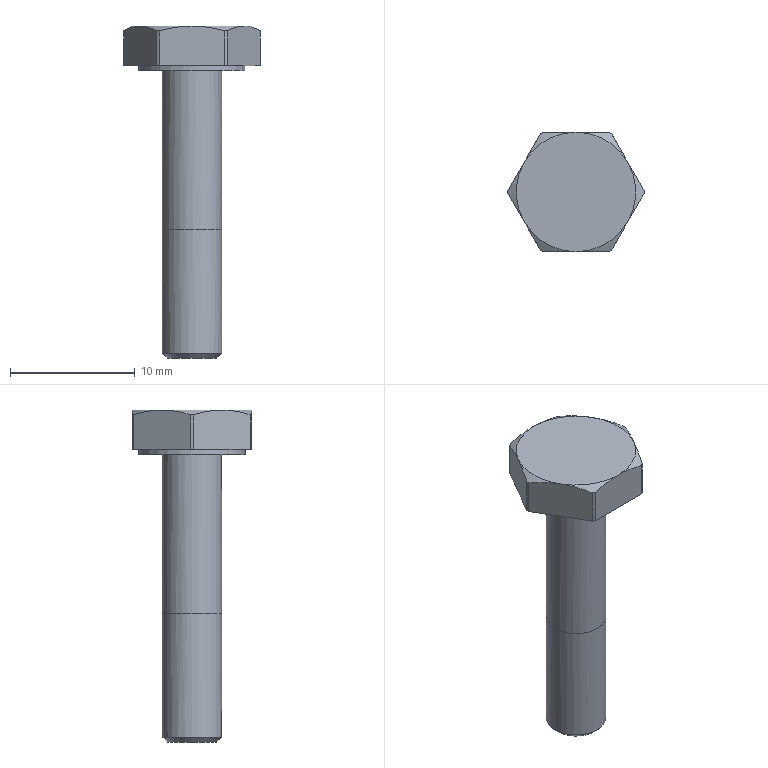Part | NX | features solid 2 | 1 solid | 26 faces | box 10.922 x 9.576 x 26.6 mm | volume 683.167 mm3 | plane 10 | cylinder 9 | cone 7 | commonest cylinder face diameters 10.922 x6 4.763 x2 8.509 x1
STEP:
#1=CARTESIAN_POINT('',(-2.381,0.,-3.581));
#2=VERTEX_POINT('',#1);
#3=CARTESIAN_POINT('',(0.,0.,-3.581));
#4=DIRECTION('',(0.,0.,-1.));
#5=DIRECTION('',(-1.,0.,0.));
#6=AXIS2_PLACEMENT_3D('',#3,#4,#5);
#7=CIRCLE('',#6,2.381);
#8=EDGE_CURVE('',#2,#2,#7,.T.);
#9=ORIENTED_EDGE('',*,*,#8,.T.);
#10=EDGE_LOOP('',(#9));
#11=FACE_BOUND('',#10,.T.);
#12=CARTESIAN_POINT('',(-2.381,0.,-16.281));
#13=VERTEX_POINT('',#12);
#14=CARTESIAN_POINT('',(-1.866,1.866,-16.281));
#15=CARTESIAN_POINT('',(-2.639,0.,-16.281));
#16=CARTESIAN_POINT('',(-1.866,-1.866,-16.281));
#17=CARTESIAN_POINT('',(0.,-2.639,-16.281));
#18=CARTESIAN_POINT('',(1.866,-1.866,-16.281));
#19=CARTESIAN_POINT('',(2.639,0.,-16.281));
#20=CARTESIAN_POINT('',(1.866,1.866,-16.281));
#21=CARTESIAN_POINT('',(0.,2.639,-16.281));
#22=CARTESIAN_POINT('',(-1.866,1.866,-16.281));
#23=CARTESIAN_POINT('',(-2.639,0.,-16.281));
#24=CARTESIAN_POINT('',(-1.866,-1.866,-16.281));
#25=B_SPLINE_CURVE_WITH_KNOTS('',3,(#14,#15,#16,#17,#18,#19,#20,#21,#22,#23,#24),.UNSPECIFIED.,.T.,.F.,(1,1,1,1,1,1,1,1,1,1,1,1,1,1,1),(-0.375,-0.25,-0.125,0.,0.125,0.25,0.375,0.5,0.625,0.75,0.875,1.,1.125,1.25,1.375),.UNSPECIFIED.);
#26=EDGE_CURVE('',#13,#13,#25,.T.);
#27=ORIENTED_EDGE('',*,*,#26,.T.);
#28=EDGE_LOOP('',(#27));
#29=FACE_BOUND('',#28,.T.);
#30=CARTESIAN_POINT('',(0.,0.,0.));
#31=DIRECTION('',(0.,0.,-1.));
#32=DIRECTION('',(-1.,0.,0.));
#33=AXIS2_PLACEMENT_3D('',#30,#31,#32);
#34=CYLINDRICAL_SURFACE('',#33,2.381);
#35=ADVANCED_FACE('',(#11,#29),#34,.T.);
#36=CARTESIAN_POINT('',(2.627,4.788,-3.175));
#37=VERTEX_POINT('',#36);
#38=CARTESIAN_POINT('',(2.833,4.669,-3.175));
#39=VERTEX_POINT('',#38);
#40=CARTESIAN_POINT('',(0.,0.,-3.175));
#41=DIRECTION('',(0.,0.,-1.));
#42=DIRECTION('',(-1.,0.,0.));
#43=AXIS2_PLACEMENT_3D('',#40,#41,#42);
#44=CIRCLE('',#43,5.461);
#45=EDGE_CURVE('',#37,#39,#44,.T.);
#46=ORIENTED_EDGE('',*,*,#45,.F.);
#47=CARTESIAN_POINT('',(2.627,4.788,-0.3886));
#48=VERTEX_POINT('',#47);
#49=CARTESIAN_POINT('',(2.627,4.788,0.));
#50=DIRECTION('',(0.,0.,-1.));
#51=VECTOR('',#50,1000.);
#52=LINE('',#49,#51);
#53=EDGE_CURVE('',#37,#48,#52,.F.);
#54=ORIENTED_EDGE('',*,*,#53,.T.);
#55=CARTESIAN_POINT('',(2.833,4.669,-0.3886));
#56=VERTEX_POINT('',#55);
#57=CARTESIAN_POINT('',(0.,0.,-0.3886));
#58=DIRECTION('',(0.,0.,-1.));
#59=DIRECTION('',(-1.,0.,0.));
#60=AXIS2_PLACEMENT_3D('',#57,#58,#59);
#61=CIRCLE('',#60,5.461);
#62=EDGE_CURVE('',#48,#56,#61,.T.);
#63=ORIENTED_EDGE('',*,*,#62,.T.);
#64=CARTESIAN_POINT('',(2.833,4.669,0.));
#65=DIRECTION('',(0.,0.,-1.));
#66=VECTOR('',#65,1000.);
#67=LINE('',#64,#66);
#68=EDGE_CURVE('',#56,#39,#67,.T.);
#69=ORIENTED_EDGE('',*,*,#68,.T.);
#70=EDGE_LOOP('',(#46,#54,#63,#69));
#71=FACE_BOUND('',#70,.T.);
#72=CARTESIAN_POINT('',(0.,0.,0.));
#73=DIRECTION('',(0.,0.,-1.));
#74=DIRECTION('',(-1.,0.,0.));
#75=AXIS2_PLACEMENT_3D('',#72,#73,#74);
#76=CYLINDRICAL_SURFACE('',#75,5.461);
#77=ADVANCED_FACE('',(#71),#76,.T.);
#78=CARTESIAN_POINT('',(-2.833,4.669,-0.3886));
#79=VERTEX_POINT('',#78);
#80=CARTESIAN_POINT('',(-2.627,4.788,-0.3886));
#81=VERTEX_POINT('',#80);
#82=CARTESIAN_POINT('',(0.,0.,-0.3886));
#83=DIRECTION('',(0.,0.,-1.));
#84=DIRECTION('',(-1.,0.,0.));
#85=AXIS2_PLACEMENT_3D('',#82,#83,#84);
#86=CIRCLE('',#85,5.461);
#87=EDGE_CURVE('',#79,#81,#86,.T.);
#88=ORIENTED_EDGE('',*,*,#87,.T.);
#89=CARTESIAN_POINT('',(-2.627,4.788,-3.175));
#90=VERTEX_POINT('',#89);
#91=CARTESIAN_POINT('',(-2.627,4.788,0.));
#92=DIRECTION('',(0.,0.,-1.));
#93=VECTOR('',#92,1000.);
#94=LINE('',#91,#93);
#95=EDGE_CURVE('',#81,#90,#94,.T.);
#96=ORIENTED_EDGE('',*,*,#95,.T.);
#97=CARTESIAN_POINT('',(-2.833,4.669,-3.175));
#98=VERTEX_POINT('',#97);
#99=CARTESIAN_POINT('',(0.,0.,-3.175));
#100=DIRECTION('',(0.,0.,-1.));
#101=DIRECTION('',(-1.,0.,0.));
#102=AXIS2_PLACEMENT_3D('',#99,#100,#101);
#103=CIRCLE('',#102,5.461);
#104=EDGE_CURVE('',#98,#90,#103,.T.);
#105=ORIENTED_EDGE('',*,*,#104,.F.);
#106=CARTESIAN_POINT('',(-2.833,4.669,0.));
#107=DIRECTION('',(0.,0.,-1.));
#108=VECTOR('',#107,1000.);
#109=LINE('',#106,#108);
#110=EDGE_CURVE('',#98,#79,#109,.F.);
#111=ORIENTED_EDGE('',*,*,#110,.T.);
#112=EDGE_LOOP('',(#88,#96,#105,#111));
#113=FACE_BOUND('',#112,.T.);
#114=CARTESIAN_POINT('',(0.,0.,0.));
#115=DIRECTION('',(0.,0.,-1.));
#116=DIRECTION('',(-1.,0.,0.));
#117=AXIS2_PLACEMENT_3D('',#114,#115,#116);
#118=CYLINDRICAL_SURFACE('',#117,5.461);
#119=ADVANCED_FACE('',(#113),#118,.T.);
#120=CARTESIAN_POINT('',(-5.46,-0.1193,-0.3886));
#121=VERTEX_POINT('',#120);
#122=CARTESIAN_POINT('',(-5.46,0.1193,-0.3886));
#123=VERTEX_POINT('',#122);
#124=CARTESIAN_POINT('',(0.,0.,-0.3886));
#125=DIRECTION('',(0.,0.,-1.));
#126=DIRECTION('',(-1.,0.,0.));
#127=AXIS2_PLACEMENT_3D('',#124,#125,#126);
#128=CIRCLE('',#127,5.461);
#129=EDGE_CURVE('',#121,#123,#128,.T.);
#130=ORIENTED_EDGE('',*,*,#129,.T.);
#131=CARTESIAN_POINT('',(-5.46,0.1193,-3.175));
#132=VERTEX_POINT('',#131);
#133=CARTESIAN_POINT('',(-5.46,0.1193,0.));
#134=DIRECTION('',(0.,0.,-1.));
#135=VECTOR('',#134,1000.);
#136=LINE('',#133,#135);
#137=EDGE_CURVE('',#123,#132,#136,.T.);
#138=ORIENTED_EDGE('',*,*,#137,.T.);
#139=CARTESIAN_POINT('',(-5.46,-0.1193,-3.175));
#140=VERTEX_POINT('',#139);
#141=CARTESIAN_POINT('',(0.,0.,-3.175));
#142=DIRECTION('',(0.,0.,-1.));
#143=DIRECTION('',(-1.,0.,0.));
#144=AXIS2_PLACEMENT_3D('',#141,#142,#143);
#145=CIRCLE('',#144,5.461);
#146=EDGE_CURVE('',#140,#132,#145,.T.);
#147=ORIENTED_EDGE('',*,*,#146,.F.);
#148=CARTESIAN_POINT('',(-5.46,-0.1193,0.));
#149=DIRECTION('',(0.,0.,-1.));
#150=VECTOR('',#149,1000.);
#151=LINE('',#148,#150);
#152=EDGE_CURVE('',#140,#121,#151,.F.);
#153=ORIENTED_EDGE('',*,*,#152,.T.);
#154=EDGE_LOOP('',(#130,#138,#147,#153));
#155=FACE_BOUND('',#154,.T.);
#156=CARTESIAN_POINT('',(0.,0.,0.));
#157=DIRECTION('',(0.,0.,-1.));
#158=DIRECTION('',(-1.,0.,0.));
#159=AXIS2_PLACEMENT_3D('',#156,#157,#158);
#160=CYLINDRICAL_SURFACE('',#159,5.461);
#161=ADVANCED_FACE('',(#155),#160,.T.);
#162=CARTESIAN_POINT('',(-2.627,-4.788,-0.3886));
#163=VERTEX_POINT('',#162);
#164=CARTESIAN_POINT('',(-2.833,-4.669,-0.3886));
#165=VERTEX_POINT('',#164);
#166=CARTESIAN_POINT('',(0.,0.,-0.3886));
#167=DIRECTION('',(0.,0.,-1.));
#168=DIRECTION('',(-1.,0.,0.));
#169=AXIS2_PLACEMENT_3D('',#166,#167,#168);
#170=CIRCLE('',#169,5.461);
#171=EDGE_CURVE('',#163,#165,#170,.T.);
#172=ORIENTED_EDGE('',*,*,#171,.T.);
#173=CARTESIAN_POINT('',(-2.833,-4.669,-3.175));
#174=VERTEX_POINT('',#173);
#175=CARTESIAN_POINT('',(-2.833,-4.669,0.));
#176=DIRECTION('',(0.,0.,-1.));
#177=VECTOR('',#176,1000.);
#178=LINE('',#175,#177);
#179=EDGE_CURVE('',#165,#174,#178,.T.);
#180=ORIENTED_EDGE('',*,*,#179,.T.);
#181=CARTESIAN_POINT('',(-2.627,-4.788,-3.175));
#182=VERTEX_POINT('',#181);
#183=CARTESIAN_POINT('',(0.,0.,-3.175));
#184=DIRECTION('',(0.,0.,-1.));
#185=DIRECTION('',(-1.,0.,0.));
#186=AXIS2_PLACEMENT_3D('',#183,#184,#185);
#187=CIRCLE('',#186,5.461);
#188=EDGE_CURVE('',#182,#174,#187,.T.);
#189=ORIENTED_EDGE('',*,*,#188,.F.);
#190=CARTESIAN_POINT('',(-2.627,-4.788,0.));
#191=DIRECTION('',(0.,0.,-1.));
#192=VECTOR('',#191,1000.);
#193=LINE('',#190,#192);
#194=EDGE_CURVE('',#182,#163,#193,.F.);
#195=ORIENTED_EDGE('',*,*,#194,.T.);
#196=EDGE_LOOP('',(#172,#180,#189,#195));
#197=FACE_BOUND('',#196,.T.);
#198=CARTESIAN_POINT('',(0.,0.,0.));
#199=DIRECTION('',(0.,0.,-1.));
#200=DIRECTION('',(-1.,0.,0.));
#201=AXIS2_PLACEMENT_3D('',#198,#199,#200);
#202=CYLINDRICAL_SURFACE('',#201,5.461);
#203=ADVANCED_FACE('',(#197),#202,.T.);
#204=CARTESIAN_POINT('',(2.833,-4.669,-0.3886));
#205=VERTEX_POINT('',#204);
#206=CARTESIAN_POINT('',(2.627,-4.788,-0.3886));
#207=VERTEX_POINT('',#206);
#208=CARTESIAN_POINT('',(0.,0.,-0.3886));
#209=DIRECTION('',(0.,0.,-1.));
#210=DIRECTION('',(-1.,0.,0.));
#211=AXIS2_PLACEMENT_3D('',#208,#209,#210);
#212=CIRCLE('',#211,5.461);
#213=EDGE_CURVE('',#205,#207,#212,.T.);
#214=ORIENTED_EDGE('',*,*,#213,.T.);
#215=CARTESIAN_POINT('',(2.627,-4.788,-3.175));
#216=VERTEX_POINT('',#215);
#217=CARTESIAN_POINT('',(2.627,-4.788,0.));
#218=DIRECTION('',(0.,0.,-1.));
#219=VECTOR('',#218,1000.);
#220=LINE('',#217,#219);
#221=EDGE_CURVE('',#207,#216,#220,.T.);
#222=ORIENTED_EDGE('',*,*,#221,.T.);
#223=CARTESIAN_POINT('',(2.833,-4.669,-3.175));
#224=VERTEX_POINT('',#223);
#225=CARTESIAN_POINT('',(0.,0.,-3.175));
#226=DIRECTION('',(0.,0.,-1.));
#227=DIRECTION('',(-1.,0.,0.));
#228=AXIS2_PLACEMENT_3D('',#225,#226,#227);
#229=CIRCLE('',#228,5.461);
#230=EDGE_CURVE('',#224,#216,#229,.T.);
#231=ORIENTED_EDGE('',*,*,#230,.F.);
#232=CARTESIAN_POINT('',(2.833,-4.669,0.));
#233=DIRECTION('',(0.,0.,-1.));
#234=VECTOR('',#233,1000.);
#235=LINE('',#232,#234);
#236=EDGE_CURVE('',#224,#205,#235,.F.);
#237=ORIENTED_EDGE('',*,*,#236,.T.);
#238=EDGE_LOOP('',(#214,#222,#231,#237));
#239=FACE_BOUND('',#238,.T.);
#240=CARTESIAN_POINT('',(0.,0.,0.));
#241=DIRECTION('',(0.,0.,-1.));
#242=DIRECTION('',(-1.,0.,0.));
#243=AXIS2_PLACEMENT_3D('',#240,#241,#242);
#244=CYLINDRICAL_SURFACE('',#243,5.461);
#245=ADVANCED_FACE('',(#239),#244,.T.);
#246=ORIENTED_EDGE('',*,*,#62,.F.);
#247=CARTESIAN_POINT('',(0.,4.788,0.));
#248=VERTEX_POINT('',#247);
#249=CARTESIAN_POINT('',(0.,4.788,0.));
#250=CARTESIAN_POINT('',(0.8868,4.788,0.));
#251=CARTESIAN_POINT('',(1.776,4.788,-0.1525));
#252=CARTESIAN_POINT('',(2.627,4.788,-0.3886));
#253=B_SPLINE_CURVE_WITH_KNOTS('',3,(#249,#250,#251,#252),.UNSPECIFIED.,.F.,.F.,(4,4),(0.007722,0.01038),.UNSPECIFIED.);
#254=EDGE_CURVE('',#48,#248,#253,.F.);
#255=ORIENTED_EDGE('',*,*,#254,.T.);
#256=CARTESIAN_POINT('',(4.146,2.394,0.));
#257=VERTEX_POINT('',#256);
#258=CARTESIAN_POINT('',(0.,0.,0.));
#259=DIRECTION('',(0.,0.,-1.));
#260=DIRECTION('',(-1.,0.,0.));
#261=AXIS2_PLACEMENT_3D('',#258,#259,#260);
#262=CIRCLE('',#261,4.788);
#263=EDGE_CURVE('',#248,#257,#262,.T.);
#264=ORIENTED_EDGE('',*,*,#263,.T.);
#265=CARTESIAN_POINT('',(4.146,2.394,0.));
#266=CARTESIAN_POINT('',(3.703,3.163,0.));
#267=CARTESIAN_POINT('',(3.262,3.925,-0.1503));
#268=CARTESIAN_POINT('',(2.833,4.669,-0.3886));
#269=B_SPLINE_CURVE_WITH_KNOTS('',3,(#265,#266,#267,#268),.UNSPECIFIED.,.F.,.F.,(4,4),(0.002655,0.005296),.UNSPECIFIED.);
#270=EDGE_CURVE('',#257,#56,#269,.T.);
#271=ORIENTED_EDGE('',*,*,#270,.T.);
#272=EDGE_LOOP('',(#246,#255,#264,#271));
#273=FACE_BOUND('',#272,.T.);
#274=CARTESIAN_POINT('',(0.,0.,-0.3886));
#275=DIRECTION('',(0.,0.,-1.));
#276=DIRECTION('',(-1.,0.,0.));
#277=AXIS2_PLACEMENT_3D('',#274,#275,#276);
#278=CONICAL_SURFACE('',#277,5.461,1.047);
#279=ADVANCED_FACE('',(#273),#278,.T.);
#280=CARTESIAN_POINT('',(-4.146,2.394,0.));
#281=VERTEX_POINT('',#280);
#282=CARTESIAN_POINT('',(0.,0.,0.));
#283=DIRECTION('',(0.,0.,-1.));
#284=DIRECTION('',(-1.,0.,0.));
#285=AXIS2_PLACEMENT_3D('',#282,#283,#284);
#286=CIRCLE('',#285,4.788);
#287=EDGE_CURVE('',#281,#248,#286,.T.);
#288=ORIENTED_EDGE('',*,*,#287,.T.);
#289=CARTESIAN_POINT('',(-2.627,4.788,-0.3886));
#290=CARTESIAN_POINT('',(-1.77,4.788,-0.1508));
#291=CARTESIAN_POINT('',(-0.8866,4.788,0.));
#292=CARTESIAN_POINT('',(0.,4.788,0.));
#293=B_SPLINE_CURVE_WITH_KNOTS('',3,(#289,#290,#291,#292),.UNSPECIFIED.,.F.,.F.,(4,4),(0.005068,0.007722),.UNSPECIFIED.);
#294=EDGE_CURVE('',#248,#81,#293,.F.);
#295=ORIENTED_EDGE('',*,*,#294,.T.);
#296=ORIENTED_EDGE('',*,*,#87,.F.);
#297=CARTESIAN_POINT('',(-2.833,4.669,-0.3886));
#298=CARTESIAN_POINT('',(-3.264,3.923,-0.1495));
#299=CARTESIAN_POINT('',(-3.7,3.167,0.));
#300=CARTESIAN_POINT('',(-4.146,2.394,0.));
#301=B_SPLINE_CURVE_WITH_KNOTS('',3,(#297,#298,#299,#300),.UNSPECIFIED.,.F.,.F.,(4,4),(0.00000074,0.002655),.UNSPECIFIED.);
#302=EDGE_CURVE('',#79,#281,#301,.T.);
#303=ORIENTED_EDGE('',*,*,#302,.T.);
#304=EDGE_LOOP('',(#288,#295,#296,#303));
#305=FACE_BOUND('',#304,.T.);
#306=CARTESIAN_POINT('',(0.,0.,-0.3886));
#307=DIRECTION('',(0.,0.,-1.));
#308=DIRECTION('',(-1.,0.,0.));
#309=AXIS2_PLACEMENT_3D('',#306,#307,#308);
#310=CONICAL_SURFACE('',#309,5.461,1.047);
#311=ADVANCED_FACE('',(#305),#310,.T.);
#312=CARTESIAN_POINT('',(-4.146,-2.394,0.));
#313=VERTEX_POINT('',#312);
#314=CARTESIAN_POINT('',(0.,0.,0.));
#315=DIRECTION('',(0.,0.,-1.));
#316=DIRECTION('',(-1.,0.,0.));
#317=AXIS2_PLACEMENT_3D('',#314,#315,#316);
#318=CIRCLE('',#317,4.788);
#319=EDGE_CURVE('',#313,#281,#318,.T.);
#320=ORIENTED_EDGE('',*,*,#319,.T.);
#321=CARTESIAN_POINT('',(-4.146,2.394,0.));
#322=CARTESIAN_POINT('',(-4.59,1.625,0.));
#323=CARTESIAN_POINT('',(-5.031,0.8625,-0.1503));
#324=CARTESIAN_POINT('',(-5.46,0.1193,-0.3886));
#325=B_SPLINE_CURVE_WITH_KNOTS('',3,(#321,#322,#323,#324),.UNSPECIFIED.,.F.,.F.,(4,4),(0.002655,0.005296),.UNSPECIFIED.);
#326=EDGE_CURVE('',#281,#123,#325,.T.);
#327=ORIENTED_EDGE('',*,*,#326,.T.);
#328=ORIENTED_EDGE('',*,*,#129,.F.);
#329=CARTESIAN_POINT('',(-5.46,-0.1193,-0.3886));
#330=CARTESIAN_POINT('',(-5.029,-0.8651,-0.1495));
#331=CARTESIAN_POINT('',(-4.593,-1.621,0.));
#332=CARTESIAN_POINT('',(-4.146,-2.394,0.));
#333=B_SPLINE_CURVE_WITH_KNOTS('',3,(#329,#330,#331,#332),.UNSPECIFIED.,.F.,.F.,(4,4),(0.00000074,0.002655),.UNSPECIFIED.);
#334=EDGE_CURVE('',#121,#313,#333,.T.);
#335=ORIENTED_EDGE('',*,*,#334,.T.);
#336=EDGE_LOOP('',(#320,#327,#328,#335));
#337=FACE_BOUND('',#336,.T.);
#338=CARTESIAN_POINT('',(0.,0.,-0.3886));
#339=DIRECTION('',(0.,0.,-1.));
#340=DIRECTION('',(-1.,0.,0.));
#341=AXIS2_PLACEMENT_3D('',#338,#339,#340);
#342=CONICAL_SURFACE('',#341,5.461,1.047);
#343=ADVANCED_FACE('',(#337),#342,.T.);
#344=CARTESIAN_POINT('',(0.,-4.788,0.));
#345=VERTEX_POINT('',#344);
#346=CARTESIAN_POINT('',(0.,0.,0.));
#347=DIRECTION('',(0.,0.,-1.));
#348=DIRECTION('',(-1.,0.,0.));
#349=AXIS2_PLACEMENT_3D('',#346,#347,#348);
#350=CIRCLE('',#349,4.788);
#351=EDGE_CURVE('',#345,#313,#350,.T.);
#352=ORIENTED_EDGE('',*,*,#351,.T.);
#353=CARTESIAN_POINT('',(-4.146,-2.394,0.));
#354=CARTESIAN_POINT('',(-3.703,-3.163,0.));
#355=CARTESIAN_POINT('',(-3.262,-3.925,-0.1503));
#356=CARTESIAN_POINT('',(-2.833,-4.669,-0.3886));
#357=B_SPLINE_CURVE_WITH_KNOTS('',3,(#353,#354,#355,#356),.UNSPECIFIED.,.F.,.F.,(4,4),(0.002655,0.005296),.UNSPECIFIED.);
#358=EDGE_CURVE('',#313,#165,#357,.T.);
#359=ORIENTED_EDGE('',*,*,#358,.T.);
#360=ORIENTED_EDGE('',*,*,#171,.F.);
#361=CARTESIAN_POINT('',(-2.627,-4.788,-0.3886));
#362=CARTESIAN_POINT('',(-1.77,-4.788,-0.1508));
#363=CARTESIAN_POINT('',(-0.8866,-4.788,0.));
#364=CARTESIAN_POINT('',(0.,-4.788,0.));
#365=B_SPLINE_CURVE_WITH_KNOTS('',3,(#361,#362,#363,#364),.UNSPECIFIED.,.F.,.F.,(4,4),(0.005068,0.007722),.UNSPECIFIED.);
#366=EDGE_CURVE('',#163,#345,#365,.T.);
#367=ORIENTED_EDGE('',*,*,#366,.T.);
#368=EDGE_LOOP('',(#352,#359,#360,#367));
#369=FACE_BOUND('',#368,.T.);
#370=CARTESIAN_POINT('',(0.,0.,-0.3886));
#371=DIRECTION('',(0.,0.,-1.));
#372=DIRECTION('',(-1.,0.,0.));
#373=AXIS2_PLACEMENT_3D('',#370,#371,#372);
#374=CONICAL_SURFACE('',#373,5.461,1.047);
#375=ADVANCED_FACE('',(#369),#374,.T.);
#376=CARTESIAN_POINT('',(4.146,-2.394,0.));
#377=VERTEX_POINT('',#376);
#378=CARTESIAN_POINT('',(0.,0.,0.));
#379=DIRECTION('',(0.,0.,-1.));
#380=DIRECTION('',(-1.,0.,0.));
#381=AXIS2_PLACEMENT_3D('',#378,#379,#380);
#382=CIRCLE('',#381,4.788);
#383=EDGE_CURVE('',#377,#345,#382,.T.);
#384=ORIENTED_EDGE('',*,*,#383,.T.);
#385=CARTESIAN_POINT('',(0.,-4.788,0.));
#386=CARTESIAN_POINT('',(0.8868,-4.788,0.));
#387=CARTESIAN_POINT('',(1.776,-4.788,-0.1525));
#388=CARTESIAN_POINT('',(2.627,-4.788,-0.3886));
#389=B_SPLINE_CURVE_WITH_KNOTS('',3,(#385,#386,#387,#388),.UNSPECIFIED.,.F.,.F.,(4,4),(0.007722,0.01038),.UNSPECIFIED.);
#390=EDGE_CURVE('',#345,#207,#389,.T.);
#391=ORIENTED_EDGE('',*,*,#390,.T.);
#392=ORIENTED_EDGE('',*,*,#213,.F.);
#393=CARTESIAN_POINT('',(2.833,-4.669,-0.3886));
#394=CARTESIAN_POINT('',(3.264,-3.923,-0.1495));
#395=CARTESIAN_POINT('',(3.7,-3.167,0.));
#396=CARTESIAN_POINT('',(4.146,-2.394,0.));
#397=B_SPLINE_CURVE_WITH_KNOTS('',3,(#393,#394,#395,#396),.UNSPECIFIED.,.F.,.F.,(4,4),(0.00000074,0.002655),.UNSPECIFIED.);
#398=EDGE_CURVE('',#205,#377,#397,.T.);
#399=ORIENTED_EDGE('',*,*,#398,.T.);
#400=EDGE_LOOP('',(#384,#391,#392,#399));
#401=FACE_BOUND('',#400,.T.);
#402=CARTESIAN_POINT('',(0.,0.,-0.3886));
#403=DIRECTION('',(0.,0.,-1.));
#404=DIRECTION('',(-1.,0.,0.));
#405=AXIS2_PLACEMENT_3D('',#402,#403,#404);
#406=CONICAL_SURFACE('',#405,5.461,1.047);
#407=ADVANCED_FACE('',(#401),#406,.T.);
#408=ORIENTED_EDGE('',*,*,#104,.T.);
#409=CARTESIAN_POINT('',(4.255,4.788,-3.175));
#410=DIRECTION('',(1.,0.,0.));
#411=VECTOR('',#410,1000.);
#412=LINE('',#409,#411);
#413=EDGE_CURVE('',#90,#37,#412,.T.);
#414=ORIENTED_EDGE('',*,*,#413,.T.);
#415=ORIENTED_EDGE('',*,*,#45,.T.);
#416=CARTESIAN_POINT('',(5.46,0.1193,-3.175));
#417=VERTEX_POINT('',#416);
#418=CARTESIAN_POINT('',(5.21,0.5517,-3.175));
#419=DIRECTION('',(0.5,-0.866,0.));
#420=VECTOR('',#419,1000.);
#421=LINE('',#418,#420);
#422=EDGE_CURVE('',#39,#417,#421,.T.);
#423=ORIENTED_EDGE('',*,*,#422,.T.);
#424=CARTESIAN_POINT('',(5.46,-0.1193,-3.175));
#425=VERTEX_POINT('',#424);
#426=CARTESIAN_POINT('',(0.,0.,-3.175));
#427=DIRECTION('',(0.,0.,-1.));
#428=DIRECTION('',(-1.,0.,0.));
#429=AXIS2_PLACEMENT_3D('',#426,#427,#428);
#430=CIRCLE('',#429,5.461);
#431=EDGE_CURVE('',#417,#425,#430,.T.);
#432=ORIENTED_EDGE('',*,*,#431,.T.);
#433=CARTESIAN_POINT('',(5.21,-0.5517,-3.175));
#434=DIRECTION('',(-0.5,-0.866,0.));
#435=VECTOR('',#434,1000.);
#436=LINE('',#433,#435);
#437=EDGE_CURVE('',#425,#224,#436,.T.);
#438=ORIENTED_EDGE('',*,*,#437,.T.);
#439=ORIENTED_EDGE('',*,*,#230,.T.);
#440=CARTESIAN_POINT('',(4.255,-4.788,-3.175));
#441=DIRECTION('',(-1.,0.,0.));
#442=VECTOR('',#441,1000.);
#443=LINE('',#440,#442);
#444=EDGE_CURVE('',#216,#182,#443,.T.);
#445=ORIENTED_EDGE('',*,*,#444,.T.);
#446=ORIENTED_EDGE('',*,*,#188,.T.);
#447=CARTESIAN_POINT('',(-3.083,-4.236,-3.175));
#448=DIRECTION('',(-0.5,0.866,0.));
#449=VECTOR('',#448,1000.);
#450=LINE('',#447,#449);
#451=EDGE_CURVE('',#174,#140,#450,.T.);
#452=ORIENTED_EDGE('',*,*,#451,.T.);
#453=ORIENTED_EDGE('',*,*,#146,.T.);
#454=CARTESIAN_POINT('',(-3.083,4.236,-3.175));
#455=DIRECTION('',(0.5,0.866,0.));
#456=VECTOR('',#455,1000.);
#457=LINE('',#454,#456);
#458=EDGE_CURVE('',#132,#98,#457,.T.);
#459=ORIENTED_EDGE('',*,*,#458,.T.);
#460=EDGE_LOOP('',(#408,#414,#415,#423,#432,#438,#439,#445,#446,#452,#453,#459));
#461=FACE_BOUND('',#460,.T.);
#462=CARTESIAN_POINT('',(-4.255,0.,-3.175));
#463=VERTEX_POINT('',#462);
#464=CARTESIAN_POINT('',(0.,0.,-3.175));
#465=DIRECTION('',(0.,0.,-1.));
#466=DIRECTION('',(-1.,0.,0.));
#467=AXIS2_PLACEMENT_3D('',#464,#465,#466);
#468=CIRCLE('',#467,4.255);
#469=EDGE_CURVE('',#463,#463,#468,.T.);
#470=ORIENTED_EDGE('',*,*,#469,.F.);
#471=EDGE_LOOP('',(#470));
#472=FACE_BOUND('',#471,.T.);
#473=CARTESIAN_POINT('',(4.255,0.,-3.175));
#474=DIRECTION('',(0.,0.,-1.));
#475=DIRECTION('',(-1.,0.,0.));
#476=AXIS2_PLACEMENT_3D('',#473,#474,#475);
#477=PLANE('',#476);
#478=ADVANCED_FACE('',(#461,#472),#477,.T.);
#479=CARTESIAN_POINT('',(5.46,0.1193,-0.3886));
#480=VERTEX_POINT('',#479);
#481=CARTESIAN_POINT('',(5.46,-0.1193,-0.3886));
#482=VERTEX_POINT('',#481);
#483=CARTESIAN_POINT('',(0.,0.,-0.3886));
#484=DIRECTION('',(0.,0.,-1.));
#485=DIRECTION('',(-1.,0.,0.));
#486=AXIS2_PLACEMENT_3D('',#483,#484,#485);
#487=CIRCLE('',#486,5.461);
#488=EDGE_CURVE('',#480,#482,#487,.T.);
#489=ORIENTED_EDGE('',*,*,#488,.T.);
#490=CARTESIAN_POINT('',(5.46,-0.1193,0.));
#491=DIRECTION('',(0.,0.,-1.));
#492=VECTOR('',#491,1000.);
#493=LINE('',#490,#492);
#494=EDGE_CURVE('',#482,#425,#493,.T.);
#495=ORIENTED_EDGE('',*,*,#494,.T.);
#496=ORIENTED_EDGE('',*,*,#431,.F.);
#497=CARTESIAN_POINT('',(5.46,0.1193,0.));
#498=DIRECTION('',(0.,0.,-1.));
#499=VECTOR('',#498,1000.);
#500=LINE('',#497,#499);
#501=EDGE_CURVE('',#417,#480,#500,.F.);
#502=ORIENTED_EDGE('',*,*,#501,.T.);
#503=EDGE_LOOP('',(#489,#495,#496,#502));
#504=FACE_BOUND('',#503,.T.);
#505=CARTESIAN_POINT('',(0.,0.,0.));
#506=DIRECTION('',(0.,0.,-1.));
#507=DIRECTION('',(-1.,0.,0.));
#508=AXIS2_PLACEMENT_3D('',#505,#506,#507);
#509=CYLINDRICAL_SURFACE('',#508,5.461);
#510=ADVANCED_FACE('',(#504),#509,.T.);
#511=CARTESIAN_POINT('',(0.,0.,0.));
#512=DIRECTION('',(0.,0.,-1.));
#513=DIRECTION('',(-1.,0.,0.));
#514=AXIS2_PLACEMENT_3D('',#511,#512,#513);
#515=CIRCLE('',#514,4.788);
#516=EDGE_CURVE('',#257,#377,#515,.T.);
#517=ORIENTED_EDGE('',*,*,#516,.T.);
#518=CARTESIAN_POINT('',(4.146,-2.394,0.));
#519=CARTESIAN_POINT('',(4.59,-1.625,0.));
#520=CARTESIAN_POINT('',(5.031,-0.8625,-0.1503));
#521=CARTESIAN_POINT('',(5.46,-0.1193,-0.3886));
#522=B_SPLINE_CURVE_WITH_KNOTS('',3,(#518,#519,#520,#521),.UNSPECIFIED.,.F.,.F.,(4,4),(0.002655,0.005296),.UNSPECIFIED.);
#523=EDGE_CURVE('',#377,#482,#522,.T.);
#524=ORIENTED_EDGE('',*,*,#523,.T.);
#525=ORIENTED_EDGE('',*,*,#488,.F.);
#526=CARTESIAN_POINT('',(5.46,0.1193,-0.3886));
#527=CARTESIAN_POINT('',(5.029,0.8651,-0.1495));
#528=CARTESIAN_POINT('',(4.593,1.621,0.));
#529=CARTESIAN_POINT('',(4.146,2.394,0.));
#530=B_SPLINE_CURVE_WITH_KNOTS('',3,(#526,#527,#528,#529),.UNSPECIFIED.,.F.,.F.,(4,4),(0.00000074,0.002655),.UNSPECIFIED.);
#531=EDGE_CURVE('',#480,#257,#530,.T.);
#532=ORIENTED_EDGE('',*,*,#531,.T.);
#533=EDGE_LOOP('',(#517,#524,#525,#532));
#534=FACE_BOUND('',#533,.T.);
#535=CARTESIAN_POINT('',(0.,0.,-0.3886));
#536=DIRECTION('',(0.,0.,-1.));
#537=DIRECTION('',(-1.,0.,0.));
#538=AXIS2_PLACEMENT_3D('',#535,#536,#537);
#539=CONICAL_SURFACE('',#538,5.461,1.047);
#540=ADVANCED_FACE('',(#534),#539,.T.);
#541=ORIENTED_EDGE('',*,*,#287,.F.);
#542=ORIENTED_EDGE('',*,*,#319,.F.);
#543=ORIENTED_EDGE('',*,*,#351,.F.);
#544=ORIENTED_EDGE('',*,*,#383,.F.);
#545=ORIENTED_EDGE('',*,*,#516,.F.);
#546=ORIENTED_EDGE('',*,*,#263,.F.);
#547=EDGE_LOOP('',(#541,#542,#543,#544,#545,#546));
#548=FACE_BOUND('',#547,.T.);
#549=CARTESIAN_POINT('',(4.788,0.,0.));
#550=DIRECTION('',(0.,0.,1.));
#551=DIRECTION('',(1.,0.,0.));
#552=AXIS2_PLACEMENT_3D('',#549,#550,#551);
#553=PLANE('',#552);
#554=ADVANCED_FACE('',(#548),#553,.T.);
#555=CARTESIAN_POINT('',(-2.,0.,-26.6));
#556=VERTEX_POINT('',#555);
#557=CARTESIAN_POINT('',(0.,0.,-26.6));
#558=DIRECTION('',(0.,0.,-1.));
#559=DIRECTION('',(-1.,0.,0.));
#560=AXIS2_PLACEMENT_3D('',#557,#558,#559);
#561=CIRCLE('',#560,2.);
#562=EDGE_CURVE('',#556,#556,#561,.T.);
#563=ORIENTED_EDGE('',*,*,#562,.T.);
#564=EDGE_LOOP('',(#563));
#565=FACE_BOUND('',#564,.T.);
#566=CARTESIAN_POINT('',(0.,0.,-26.6));
#567=DIRECTION('',(0.,0.,-1.));
#568=DIRECTION('',(-1.,0.,0.));
#569=AXIS2_PLACEMENT_3D('',#566,#567,#568);
#570=PLANE('',#569);
#571=ADVANCED_FACE('',(#565),#570,.T.);
#572=CARTESIAN_POINT('',(-2.381,0.,-26.219));
#573=VERTEX_POINT('',#572);
#574=CARTESIAN_POINT('',(0.,0.,-26.219));
#575=DIRECTION('',(0.,0.,-1.));
#576=DIRECTION('',(-1.,0.,0.));
#577=AXIS2_PLACEMENT_3D('',#574,#575,#576);
#578=CIRCLE('',#577,2.381);
#579=EDGE_CURVE('',#573,#573,#578,.T.);
#580=ORIENTED_EDGE('',*,*,#579,.T.);
#581=EDGE_LOOP('',(#580));
#582=FACE_BOUND('',#581,.T.);
#583=ORIENTED_EDGE('',*,*,#562,.F.);
#584=EDGE_LOOP('',(#583));
#585=FACE_BOUND('',#584,.T.);
#586=CARTESIAN_POINT('',(0.,0.,-26.6));
#587=DIRECTION('',(0.,0.,1.));
#588=DIRECTION('',(1.,0.,0.));
#589=AXIS2_PLACEMENT_3D('',#586,#587,#588);
#590=CONICAL_SURFACE('',#589,2.,0.7854);
#591=ADVANCED_FACE('',(#582,#585),#590,.T.);
#592=ORIENTED_EDGE('',*,*,#26,.F.);
#593=EDGE_LOOP('',(#592));
#594=FACE_BOUND('',#593,.T.);
#595=ORIENTED_EDGE('',*,*,#579,.F.);
#596=EDGE_LOOP('',(#595));
#597=FACE_BOUND('',#596,.T.);
#598=CARTESIAN_POINT('',(0.,0.,0.));
#599=DIRECTION('',(0.,0.,-1.));
#600=DIRECTION('',(-1.,0.,0.));
#601=AXIS2_PLACEMENT_3D('',#598,#599,#600);
#602=CYLINDRICAL_SURFACE('',#601,2.381);
#603=ADVANCED_FACE('',(#594,#597),#602,.T.);
#604=CARTESIAN_POINT('',(-4.255,0.,-3.581));
#605=VERTEX_POINT('',#604);
#606=CARTESIAN_POINT('',(0.,0.,-3.581));
#607=DIRECTION('',(0.,0.,-1.));
#608=DIRECTION('',(-1.,0.,0.));
#609=AXIS2_PLACEMENT_3D('',#606,#607,#608);
#610=CIRCLE('',#609,4.255);
#611=EDGE_CURVE('',#605,#605,#610,.T.);
#612=ORIENTED_EDGE('',*,*,#611,.T.);
#613=EDGE_LOOP('',(#612));
#614=FACE_BOUND('',#613,.T.);
#615=ORIENTED_EDGE('',*,*,#8,.F.);
#616=EDGE_LOOP('',(#615));
#617=FACE_BOUND('',#616,.T.);
#618=CARTESIAN_POINT('',(2.381,0.,-3.581));
#619=DIRECTION('',(0.,0.,-1.));
#620=DIRECTION('',(-1.,0.,0.));
#621=AXIS2_PLACEMENT_3D('',#618,#619,#620);
#622=PLANE('',#621);
#623=ADVANCED_FACE('',(#614,#617),#622,.T.);
#624=ORIENTED_EDGE('',*,*,#469,.T.);
#625=EDGE_LOOP('',(#624));
#626=FACE_BOUND('',#625,.T.);
#627=ORIENTED_EDGE('',*,*,#611,.F.);
#628=EDGE_LOOP('',(#627));
#629=FACE_BOUND('',#628,.T.);
#630=CARTESIAN_POINT('',(0.,0.,0.));
#631=DIRECTION('',(0.,0.,-1.));
#632=DIRECTION('',(-1.,0.,0.));
#633=AXIS2_PLACEMENT_3D('',#630,#631,#632);
#634=CYLINDRICAL_SURFACE('',#633,4.255);
#635=ADVANCED_FACE('',(#626,#629),#634,.T.);
#636=ORIENTED_EDGE('',*,*,#422,.F.);
#637=ORIENTED_EDGE('',*,*,#68,.F.);
#638=ORIENTED_EDGE('',*,*,#270,.F.);
#639=ORIENTED_EDGE('',*,*,#531,.F.);
#640=ORIENTED_EDGE('',*,*,#501,.F.);
#641=EDGE_LOOP('',(#636,#637,#638,#639,#640));
#642=FACE_BOUND('',#641,.T.);
#643=CARTESIAN_POINT('',(5.529,0.,-29.26));
#644=DIRECTION('',(0.866,0.5,0.));
#645=DIRECTION('',(-0.5,0.866,0.));
#646=AXIS2_PLACEMENT_3D('',#643,#644,#645);
#647=PLANE('',#646);
#648=ADVANCED_FACE('',(#642),#647,.T.);
#649=ORIENTED_EDGE('',*,*,#437,.F.);
#650=ORIENTED_EDGE('',*,*,#494,.F.);
#651=ORIENTED_EDGE('',*,*,#523,.F.);
#652=ORIENTED_EDGE('',*,*,#398,.F.);
#653=ORIENTED_EDGE('',*,*,#236,.F.);
#654=EDGE_LOOP('',(#649,#650,#651,#652,#653));
#655=FACE_BOUND('',#654,.T.);
#656=CARTESIAN_POINT('',(2.764,-4.788,-29.26));
#657=DIRECTION('',(0.866,-0.5,0.));
#658=DIRECTION('',(0.5,0.866,0.));
#659=AXIS2_PLACEMENT_3D('',#656,#657,#658);
#660=PLANE('',#659);
#661=ADVANCED_FACE('',(#655),#660,.T.);
#662=ORIENTED_EDGE('',*,*,#444,.F.);
#663=ORIENTED_EDGE('',*,*,#221,.F.);
#664=ORIENTED_EDGE('',*,*,#390,.F.);
#665=ORIENTED_EDGE('',*,*,#366,.F.);
#666=ORIENTED_EDGE('',*,*,#194,.F.);
#667=EDGE_LOOP('',(#662,#663,#664,#665,#666));
#668=FACE_BOUND('',#667,.T.);
#669=CARTESIAN_POINT('',(-2.764,-4.788,-29.26));
#670=DIRECTION('',(0.,-1.,0.));
#671=DIRECTION('',(0.,0.,-1.));
#672=AXIS2_PLACEMENT_3D('',#669,#670,#671);
#673=PLANE('',#672);
#674=ADVANCED_FACE('',(#668),#673,.T.);
#675=ORIENTED_EDGE('',*,*,#451,.F.);
#676=ORIENTED_EDGE('',*,*,#179,.F.);
#677=ORIENTED_EDGE('',*,*,#358,.F.);
#678=ORIENTED_EDGE('',*,*,#334,.F.);
#679=ORIENTED_EDGE('',*,*,#152,.F.);
#680=EDGE_LOOP('',(#675,#676,#677,#678,#679));
#681=FACE_BOUND('',#680,.T.);
#682=CARTESIAN_POINT('',(-5.529,0.,-29.26));
#683=DIRECTION('',(-0.866,-0.5,0.));
#684=DIRECTION('',(0.5,-0.866,0.));
#685=AXIS2_PLACEMENT_3D('',#682,#683,#684);
#686=PLANE('',#685);
#687=ADVANCED_FACE('',(#681),#686,.T.);
#688=ORIENTED_EDGE('',*,*,#458,.F.);
#689=ORIENTED_EDGE('',*,*,#137,.F.);
#690=ORIENTED_EDGE('',*,*,#326,.F.);
#691=ORIENTED_EDGE('',*,*,#302,.F.);
#692=ORIENTED_EDGE('',*,*,#110,.F.);
#693=EDGE_LOOP('',(#688,#689,#690,#691,#692));
#694=FACE_BOUND('',#693,.T.);
#695=CARTESIAN_POINT('',(-2.764,4.788,-29.26));
#696=DIRECTION('',(-0.866,0.5,0.));
#697=DIRECTION('',(-0.5,-0.866,0.));
#698=AXIS2_PLACEMENT_3D('',#695,#696,#697);
#699=PLANE('',#698);
#700=ADVANCED_FACE('',(#694),#699,.T.);
#701=ORIENTED_EDGE('',*,*,#413,.F.);
#702=ORIENTED_EDGE('',*,*,#95,.F.);
#703=ORIENTED_EDGE('',*,*,#294,.F.);
#704=ORIENTED_EDGE('',*,*,#254,.F.);
#705=ORIENTED_EDGE('',*,*,#53,.F.);
#706=EDGE_LOOP('',(#701,#702,#703,#704,#705));
#707=FACE_BOUND('',#706,.T.);
#708=CARTESIAN_POINT('',(2.764,4.788,-29.26));
#709=DIRECTION('',(0.,1.,0.));
#710=DIRECTION('',(0.,0.,1.));
#711=AXIS2_PLACEMENT_3D('',#708,#709,#710);
#712=PLANE('',#711);
#713=ADVANCED_FACE('',(#707),#712,.T.);
#714=CLOSED_SHELL('',(#35,#77,#119,#161,#203,#245,#279,#311,#343,#375,#407,#478,#510,#540,#554,#571,#591,#603,#623,#635,#648,#661,#674,#687,#700,#713));
#715=MANIFOLD_SOLID_BREP('',#714);
#716=(LENGTH_UNIT()NAMED_UNIT(*)SI_UNIT(.MILLI.,.METRE.));
#717=UNCERTAINTY_MEASURE_WITH_UNIT(LENGTH_MEASURE(0.0508),#716,'','');
#718=(NAMED_UNIT(*)PLANE_ANGLE_UNIT()SI_UNIT($,.RADIAN.));
#719=(NAMED_UNIT(*)SI_UNIT($,.STERADIAN.)SOLID_ANGLE_UNIT());
#720=(GEOMETRIC_REPRESENTATION_CONTEXT(3)GLOBAL_UNCERTAINTY_ASSIGNED_CONTEXT((#717))GLOBAL_UNIT_ASSIGNED_CONTEXT((#716,#718,#719))REPRESENTATION_CONTEXT('',''));
#721=ADVANCED_BREP_SHAPE_REPRESENTATION('',(#715),#720);